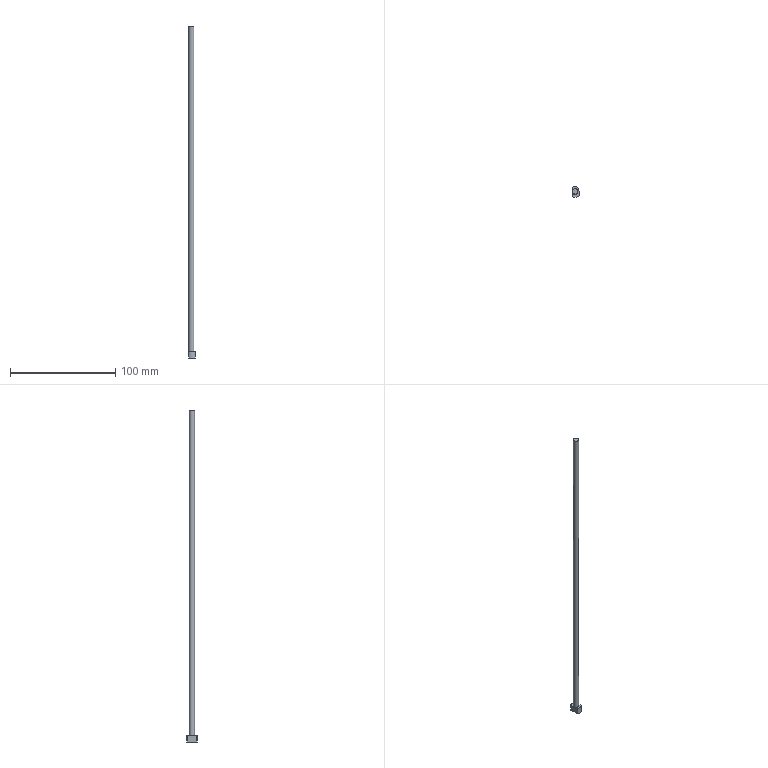Part | STEP file | 车灯-后视镜_id402_x_t | 1 solid | 8 faces | box 6.332 x 10 x 315.5 mm | volume 6416 mm3 | plane 5 | cylinder 3 | commonest cylinder face diameters 10 x2 5 x1
STEP:
#1=CARTESIAN_POINT('',(-24.5,-20.67,-249.5));
#2=VERTEX_POINT('',#1);
#3=CARTESIAN_POINT('',(-24.5,-20.67,-255.5));
#4=VERTEX_POINT('',#3);
#5=CARTESIAN_POINT('',(-24.5,-20.67,-255.5));
#6=DIRECTION('',(0.,0.,-1.));
#7=VECTOR('',#6,1.);
#8=LINE('',#5,#7);
#9=EDGE_CURVE('',#2,#4,#8,.T.);
#10=ORIENTED_EDGE('',*,*,#9,.F.);
#11=CARTESIAN_POINT('',(-18.653,-21.286,-249.5));
#12=VERTEX_POINT('',#11);
#13=CARTESIAN_POINT('',(-22.,-25.,-249.5));
#14=DIRECTION('',(0.,0.,-1.));
#15=DIRECTION('',(-1.,0.,0.));
#16=AXIS2_PLACEMENT_3D('',#13,#14,#15);
#17=CIRCLE('',#16,5.);
#18=EDGE_CURVE('',#2,#12,#17,.T.);
#19=ORIENTED_EDGE('',*,*,#18,.T.);
#20=CARTESIAN_POINT('',(-18.653,-21.286,-255.5));
#21=VERTEX_POINT('',#20);
#22=CARTESIAN_POINT('',(-18.653,-21.286,-255.5));
#23=DIRECTION('',(0.,0.,1.));
#24=VECTOR('',#23,1.);
#25=LINE('',#22,#24);
#26=EDGE_CURVE('',#21,#12,#25,.T.);
#27=ORIENTED_EDGE('',*,*,#26,.F.);
#28=CARTESIAN_POINT('',(-22.,-25.,-255.5));
#29=DIRECTION('',(0.,0.,1.));
#30=DIRECTION('',(1.,0.,0.));
#31=AXIS2_PLACEMENT_3D('',#28,#29,#30);
#32=CIRCLE('',#31,5.);
#33=EDGE_CURVE('',#21,#4,#32,.T.);
#34=ORIENTED_EDGE('',*,*,#33,.T.);
#35=EDGE_LOOP('',(#10,#19,#27,#34));
#36=FACE_OUTER_BOUND('',#35,.T.);
#37=CARTESIAN_POINT('',(-22.,-25.,-255.5));
#38=DIRECTION('',(0.,0.,1.));
#39=DIRECTION('',(1.,0.,0.));
#40=AXIS2_PLACEMENT_3D('',#37,#38,#39);
#41=CYLINDRICAL_SURFACE('',#40,5.);
#42=ADVANCED_FACE('',(#36),#41,.T.);
#43=CARTESIAN_POINT('',(-24.5,-25.,60.));
#44=VERTEX_POINT('',#43);
#45=CARTESIAN_POINT('',(-22.,-25.,60.));
#46=DIRECTION('',(0.,0.,-1.));
#47=DIRECTION('',(-1.,0.,0.));
#48=AXIS2_PLACEMENT_3D('',#45,#46,#47);
#49=CIRCLE('',#48,2.5);
#50=EDGE_CURVE('',#44,#44,#49,.T.);
#51=ORIENTED_EDGE('',*,*,#50,.F.);
#52=EDGE_LOOP('',(#51));
#53=FACE_OUTER_BOUND('',#52,.T.);
#54=CARTESIAN_POINT('',(-22.,-25.,60.));
#55=DIRECTION('',(0.,0.,1.));
#56=DIRECTION('',(1.,0.,0.));
#57=AXIS2_PLACEMENT_3D('',#54,#55,#56);
#58=PLANE('',#57);
#59=ADVANCED_FACE('',(#53),#58,.T.);
#60=CARTESIAN_POINT('',(-24.5,-25.,-249.5));
#61=VERTEX_POINT('',#60);
#62=CARTESIAN_POINT('',(-22.,-25.,-249.5));
#63=DIRECTION('',(0.,0.,-1.));
#64=DIRECTION('',(1.,0.,0.));
#65=AXIS2_PLACEMENT_3D('',#62,#63,#64);
#66=CIRCLE('',#65,2.5);
#67=EDGE_CURVE('',#61,#61,#66,.T.);
#68=ORIENTED_EDGE('',*,*,#67,.F.);
#69=EDGE_LOOP('',(#68));
#70=FACE_BOUND('',#69,.T.);
#71=ORIENTED_EDGE('',*,*,#50,.T.);
#72=EDGE_LOOP('',(#71));
#73=FACE_BOUND('',#72,.T.);
#74=CARTESIAN_POINT('',(-22.,-25.,-190.));
#75=DIRECTION('',(0.,0.,1.));
#76=DIRECTION('',(1.,0.,0.));
#77=AXIS2_PLACEMENT_3D('',#74,#75,#76);
#78=CYLINDRICAL_SURFACE('',#77,2.5);
#79=ADVANCED_FACE('',(#70,#73),#78,.T.);
#80=CARTESIAN_POINT('',(-24.5,-29.33,-249.5));
#81=VERTEX_POINT('',#80);
#82=CARTESIAN_POINT('',(-24.5,-25.,-249.5));
#83=DIRECTION('',(0.,1.,0.));
#84=VECTOR('',#83,1.);
#85=LINE('',#82,#84);
#86=EDGE_CURVE('',#81,#61,#85,.T.);
#87=ORIENTED_EDGE('',*,*,#86,.F.);
#88=CARTESIAN_POINT('',(-18.168,-28.212,-249.5));
#89=VERTEX_POINT('',#88);
#90=CARTESIAN_POINT('',(-22.,-25.,-249.5));
#91=DIRECTION('',(0.,0.,-1.));
#92=DIRECTION('',(-1.,0.,0.));
#93=AXIS2_PLACEMENT_3D('',#90,#91,#92);
#94=CIRCLE('',#93,5.);
#95=EDGE_CURVE('',#89,#81,#94,.T.);
#96=ORIENTED_EDGE('',*,*,#95,.F.);
#97=CARTESIAN_POINT('',(-18.411,-24.749,-249.5));
#98=DIRECTION('',(0.06976,-0.9976,0.));
#99=VECTOR('',#98,1.);
#100=LINE('',#97,#99);
#101=EDGE_CURVE('',#12,#89,#100,.T.);
#102=ORIENTED_EDGE('',*,*,#101,.F.);
#103=ORIENTED_EDGE('',*,*,#18,.F.);
#104=CARTESIAN_POINT('',(-24.5,-25.,-249.5));
#105=DIRECTION('',(0.,1.,0.));
#106=VECTOR('',#105,1.);
#107=LINE('',#104,#106);
#108=EDGE_CURVE('',#61,#2,#107,.T.);
#109=ORIENTED_EDGE('',*,*,#108,.F.);
#110=ORIENTED_EDGE('',*,*,#67,.T.);
#111=EDGE_LOOP('',(#87,#96,#102,#103,#109,#110));
#112=FACE_OUTER_BOUND('',#111,.T.);
#113=CARTESIAN_POINT('',(-22.,-25.,-249.5));
#114=DIRECTION('',(0.,0.,1.));
#115=DIRECTION('',(1.,0.,0.));
#116=AXIS2_PLACEMENT_3D('',#113,#114,#115);
#117=PLANE('',#116);
#118=ADVANCED_FACE('',(#112),#117,.T.);
#119=CARTESIAN_POINT('',(-24.5,-29.33,-255.5));
#120=VERTEX_POINT('',#119);
#121=CARTESIAN_POINT('',(-24.5,-29.33,-255.5));
#122=DIRECTION('',(0.,0.,1.));
#123=VECTOR('',#122,1.);
#124=LINE('',#121,#123);
#125=EDGE_CURVE('',#120,#81,#124,.T.);
#126=ORIENTED_EDGE('',*,*,#125,.F.);
#127=CARTESIAN_POINT('',(-18.168,-28.212,-255.5));
#128=VERTEX_POINT('',#127);
#129=CARTESIAN_POINT('',(-22.,-25.,-255.5));
#130=DIRECTION('',(0.,0.,1.));
#131=DIRECTION('',(1.,0.,0.));
#132=AXIS2_PLACEMENT_3D('',#129,#130,#131);
#133=CIRCLE('',#132,5.);
#134=EDGE_CURVE('',#120,#128,#133,.T.);
#135=ORIENTED_EDGE('',*,*,#134,.T.);
#136=CARTESIAN_POINT('',(-18.168,-28.212,-249.5));
#137=DIRECTION('',(0.,0.,-1.));
#138=VECTOR('',#137,1.);
#139=LINE('',#136,#138);
#140=EDGE_CURVE('',#89,#128,#139,.T.);
#141=ORIENTED_EDGE('',*,*,#140,.F.);
#142=ORIENTED_EDGE('',*,*,#95,.T.);
#143=EDGE_LOOP('',(#126,#135,#141,#142));
#144=FACE_OUTER_BOUND('',#143,.T.);
#145=CARTESIAN_POINT('',(-22.,-25.,-255.5));
#146=DIRECTION('',(0.,0.,1.));
#147=DIRECTION('',(1.,0.,0.));
#148=AXIS2_PLACEMENT_3D('',#145,#146,#147);
#149=CYLINDRICAL_SURFACE('',#148,5.);
#150=ADVANCED_FACE('',(#144),#149,.T.);
#151=CARTESIAN_POINT('',(-24.5,-25.,-255.5));
#152=DIRECTION('',(0.,-1.,0.));
#153=VECTOR('',#152,1.);
#154=LINE('',#151,#153);
#155=EDGE_CURVE('',#4,#120,#154,.T.);
#156=ORIENTED_EDGE('',*,*,#155,.F.);
#157=ORIENTED_EDGE('',*,*,#33,.F.);
#158=CARTESIAN_POINT('',(-18.411,-24.749,-255.5));
#159=DIRECTION('',(-0.06976,0.9976,0.));
#160=VECTOR('',#159,1.);
#161=LINE('',#158,#160);
#162=EDGE_CURVE('',#128,#21,#161,.T.);
#163=ORIENTED_EDGE('',*,*,#162,.F.);
#164=ORIENTED_EDGE('',*,*,#134,.F.);
#165=EDGE_LOOP('',(#156,#157,#163,#164));
#166=FACE_OUTER_BOUND('',#165,.T.);
#167=CARTESIAN_POINT('',(-22.,-25.,-255.5));
#168=DIRECTION('',(0.,0.,-1.));
#169=DIRECTION('',(-1.,0.,0.));
#170=AXIS2_PLACEMENT_3D('',#167,#168,#169);
#171=PLANE('',#170);
#172=ADVANCED_FACE('',(#166),#171,.T.);
#173=ORIENTED_EDGE('',*,*,#101,.T.);
#174=ORIENTED_EDGE('',*,*,#140,.T.);
#175=ORIENTED_EDGE('',*,*,#162,.T.);
#176=ORIENTED_EDGE('',*,*,#26,.T.);
#177=EDGE_LOOP('',(#173,#174,#175,#176));
#178=FACE_OUTER_BOUND('',#177,.T.);
#179=CARTESIAN_POINT('',(-17.731,-34.464,-255.5));
#180=DIRECTION('',(-0.9976,-0.06976,0.));
#181=DIRECTION('',(0.06976,-0.9976,0.));
#182=AXIS2_PLACEMENT_3D('',#179,#180,#181);
#183=PLANE('',#182);
#184=ADVANCED_FACE('',(#178),#183,.F.);
#185=ORIENTED_EDGE('',*,*,#86,.T.);
#186=ORIENTED_EDGE('',*,*,#108,.T.);
#187=ORIENTED_EDGE('',*,*,#9,.T.);
#188=ORIENTED_EDGE('',*,*,#155,.T.);
#189=ORIENTED_EDGE('',*,*,#125,.T.);
#190=EDGE_LOOP('',(#185,#186,#187,#188,#189));
#191=FACE_OUTER_BOUND('',#190,.T.);
#192=CARTESIAN_POINT('',(-24.5,-25.,-249.5));
#193=DIRECTION('',(1.,0.,0.));
#194=DIRECTION('',(0.,0.,-1.));
#195=AXIS2_PLACEMENT_3D('',#192,#193,#194);
#196=PLANE('',#195);
#197=ADVANCED_FACE('',(#191),#196,.F.);
#198=CLOSED_SHELL('',(#42,#59,#79,#118,#150,#172,#184,#197));
#199=MANIFOLD_SOLID_BREP('',#198);
#200=(LENGTH_UNIT()NAMED_UNIT(*)SI_UNIT(.MILLI.,.METRE.));
#201=UNCERTAINTY_MEASURE_WITH_UNIT(LENGTH_MEASURE(0.00002),#200,'','');
#202=(NAMED_UNIT(*)PLANE_ANGLE_UNIT()SI_UNIT($,.RADIAN.));
#203=PLANE_ANGLE_MEASURE_WITH_UNIT(PLANE_ANGLE_MEASURE(0.01745),#202);
#204=DIMENSIONAL_EXPONENTS(0.,0.,0.,0.,0.,0.,0.);
#205=(CONVERSION_BASED_UNIT('DEGREE',#203)NAMED_UNIT(#204)PLANE_ANGLE_UNIT());
#206=(NAMED_UNIT(*)SI_UNIT($,.STERADIAN.)SOLID_ANGLE_UNIT());
#207=(GEOMETRIC_REPRESENTATION_CONTEXT(3)GLOBAL_UNCERTAINTY_ASSIGNED_CONTEXT((#201))GLOBAL_UNIT_ASSIGNED_CONTEXT((#200,#205,#206))REPRESENTATION_CONTEXT('',''));
#208=ADVANCED_BREP_SHAPE_REPRESENTATION('',(#199),#207);